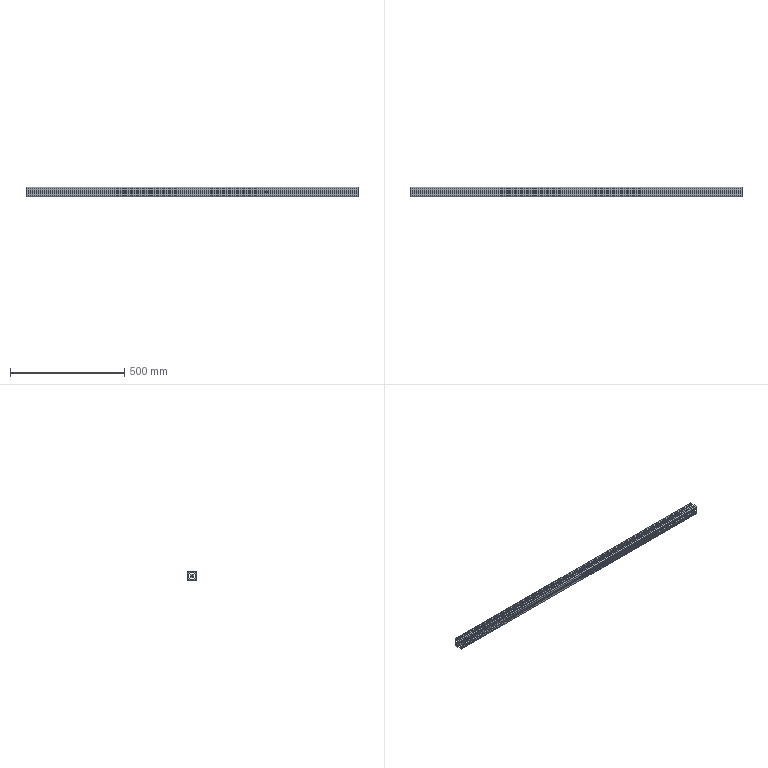Part | 1 solid | 108 faces | box 1450 x 40 x 40 mm | volume 835447 mm3 | plane 94 | cylinder 14 | commonest cylinder face diameters 5 x4 6.8 x4 9 x4 8.2 x2